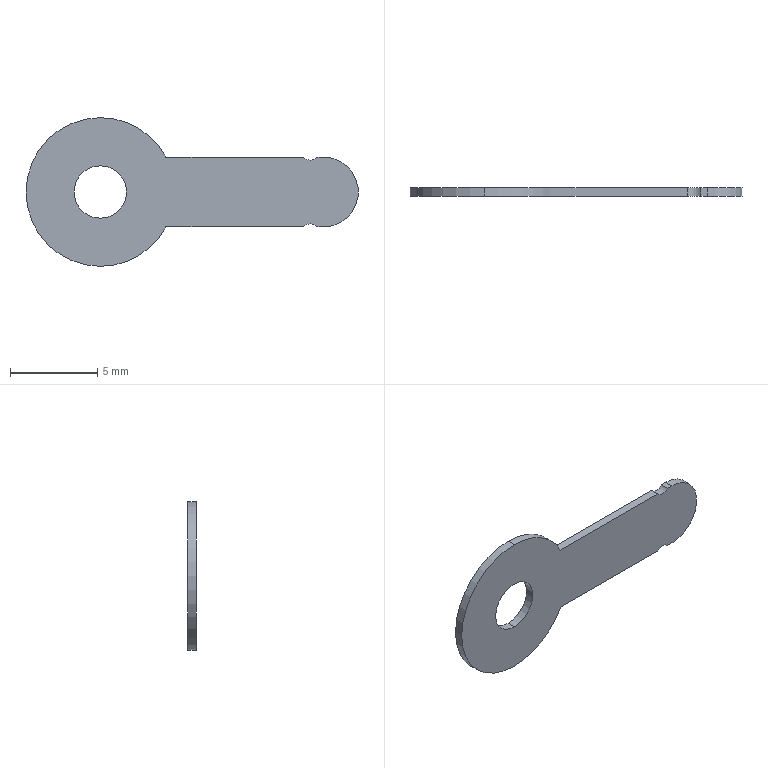Part | SolidWorks | features Extrusion 1, ICE 1 | 1 solid | 15 faces | box 19 x 0.5 x 8.5 mm | volume 45.209 mm3 | cylinder 9 | plane 6 | commonest cylinder face diameters 1 x3 8.5 x3 3 x2 4 x1
STEP:
#1=CARTESIAN_POINT('',(12.,0.,-1.82));
#2=VERTEX_POINT('',#1);
#3=CARTESIAN_POINT('',(12.384,0.,-2.));
#4=VERTEX_POINT('',#3);
#5=CARTESIAN_POINT('',(12.,0.,-2.32));
#6=DIRECTION('',(0.,1.,0.));
#7=DIRECTION('',(0.,0.,1.));
#8=AXIS2_PLACEMENT_3D('',#5,#6,#7);
#9=CIRCLE('',#8,0.5);
#10=EDGE_CURVE('',#2,#4,#9,.T.);
#11=ORIENTED_EDGE('',*,*,#10,.F.);
#12=CARTESIAN_POINT('',(12.,0.5,-1.82));
#13=VERTEX_POINT('',#12);
#14=CARTESIAN_POINT('',(12.,0.,-1.82));
#15=DIRECTION('',(0.,1.,0.));
#16=VECTOR('',#15,1000.);
#17=LINE('',#14,#16);
#18=EDGE_CURVE('',#2,#13,#17,.T.);
#19=ORIENTED_EDGE('',*,*,#18,.T.);
#20=CARTESIAN_POINT('',(12.384,0.5,-2.));
#21=VERTEX_POINT('',#20);
#22=CARTESIAN_POINT('',(12.,0.5,-2.32));
#23=DIRECTION('',(0.,1.,0.));
#24=DIRECTION('',(0.,0.,1.));
#25=AXIS2_PLACEMENT_3D('',#22,#23,#24);
#26=CIRCLE('',#25,0.5);
#27=EDGE_CURVE('',#13,#21,#26,.T.);
#28=ORIENTED_EDGE('',*,*,#27,.T.);
#29=CARTESIAN_POINT('',(12.384,0.,-2.));
#30=DIRECTION('',(0.,1.,0.));
#31=VECTOR('',#30,1000.);
#32=LINE('',#29,#31);
#33=EDGE_CURVE('',#4,#21,#32,.T.);
#34=ORIENTED_EDGE('',*,*,#33,.F.);
#35=EDGE_LOOP('',(#11,#19,#28,#34));
#36=FACE_OUTER_BOUND('',#35,.T.);
#37=CARTESIAN_POINT('',(12.,0.,-2.32));
#38=DIRECTION('',(0.,1.,0.));
#39=DIRECTION('',(0.,0.,1.));
#40=AXIS2_PLACEMENT_3D('',#37,#38,#39);
#41=CYLINDRICAL_SURFACE('',#40,0.5);
#42=ADVANCED_FACE('',(#36),#41,.F.);
#43=CARTESIAN_POINT('',(0.,0.5,-1.5));
#44=VERTEX_POINT('',#43);
#45=CARTESIAN_POINT('',(0.,0.5,1.5));
#46=VERTEX_POINT('',#45);
#47=CARTESIAN_POINT('',(0.,0.5,0.));
#48=DIRECTION('',(0.,1.,0.));
#49=DIRECTION('',(0.,0.,1.));
#50=AXIS2_PLACEMENT_3D('',#47,#48,#49);
#51=CIRCLE('',#50,1.5);
#52=EDGE_CURVE('',#44,#46,#51,.T.);
#53=ORIENTED_EDGE('',*,*,#52,.T.);
#54=CARTESIAN_POINT('',(0.,0.,1.5));
#55=VERTEX_POINT('',#54);
#56=CARTESIAN_POINT('',(0.,0.5,1.5));
#57=DIRECTION('',(0.,-1.,0.));
#58=VECTOR('',#57,1000.);
#59=LINE('',#56,#58);
#60=EDGE_CURVE('',#46,#55,#59,.T.);
#61=ORIENTED_EDGE('',*,*,#60,.T.);
#62=CARTESIAN_POINT('',(0.,0.,-1.5));
#63=VERTEX_POINT('',#62);
#64=CARTESIAN_POINT('',(0.,0.,0.));
#65=DIRECTION('',(0.,1.,0.));
#66=DIRECTION('',(0.,0.,1.));
#67=AXIS2_PLACEMENT_3D('',#64,#65,#66);
#68=CIRCLE('',#67,1.5);
#69=EDGE_CURVE('',#63,#55,#68,.T.);
#70=ORIENTED_EDGE('',*,*,#69,.F.);
#71=CARTESIAN_POINT('',(0.,0.5,-1.5));
#72=DIRECTION('',(0.,-1.,0.));
#73=VECTOR('',#72,1000.);
#74=LINE('',#71,#73);
#75=EDGE_CURVE('',#44,#63,#74,.T.);
#76=ORIENTED_EDGE('',*,*,#75,.F.);
#77=EDGE_LOOP('',(#53,#61,#70,#76));
#78=FACE_OUTER_BOUND('',#77,.T.);
#79=CARTESIAN_POINT('',(0.,0.5,0.));
#80=DIRECTION('',(0.,-1.,0.));
#81=DIRECTION('',(0.,0.,-1.));
#82=AXIS2_PLACEMENT_3D('',#79,#80,#81);
#83=CYLINDRICAL_SURFACE('',#82,1.5);
#84=ADVANCED_FACE('',(#78),#83,.F.);
#85=CARTESIAN_POINT('',(0.,0.5,4.25));
#86=VERTEX_POINT('',#85);
#87=CARTESIAN_POINT('',(3.75,0.5,2.));
#88=VERTEX_POINT('',#87);
#89=CARTESIAN_POINT('',(0.,0.5,0.));
#90=DIRECTION('',(0.,1.,0.));
#91=DIRECTION('',(0.,0.,1.));
#92=AXIS2_PLACEMENT_3D('',#89,#90,#91);
#93=CIRCLE('',#92,4.25);
#94=EDGE_CURVE('',#86,#88,#93,.T.);
#95=ORIENTED_EDGE('',*,*,#94,.F.);
#96=CARTESIAN_POINT('',(0.,0.,4.25));
#97=VERTEX_POINT('',#96);
#98=CARTESIAN_POINT('',(0.,0.5,4.25));
#99=DIRECTION('',(0.,-1.,0.));
#100=VECTOR('',#99,1000.);
#101=LINE('',#98,#100);
#102=EDGE_CURVE('',#86,#97,#101,.T.);
#103=ORIENTED_EDGE('',*,*,#102,.T.);
#104=CARTESIAN_POINT('',(3.75,0.,2.));
#105=VERTEX_POINT('',#104);
#106=CARTESIAN_POINT('',(0.,0.,0.));
#107=DIRECTION('',(0.,1.,0.));
#108=DIRECTION('',(0.,0.,1.));
#109=AXIS2_PLACEMENT_3D('',#106,#107,#108);
#110=CIRCLE('',#109,4.25);
#111=EDGE_CURVE('',#97,#105,#110,.T.);
#112=ORIENTED_EDGE('',*,*,#111,.T.);
#113=CARTESIAN_POINT('',(3.75,0.5,2.));
#114=DIRECTION('',(0.,-1.,0.));
#115=VECTOR('',#114,1000.);
#116=LINE('',#113,#115);
#117=EDGE_CURVE('',#88,#105,#116,.T.);
#118=ORIENTED_EDGE('',*,*,#117,.F.);
#119=EDGE_LOOP('',(#95,#103,#112,#118));
#120=FACE_OUTER_BOUND('',#119,.T.);
#121=CARTESIAN_POINT('',(0.,0.5,0.));
#122=DIRECTION('',(0.,-1.,0.));
#123=DIRECTION('',(0.,0.,-1.));
#124=AXIS2_PLACEMENT_3D('',#121,#122,#123);
#125=CYLINDRICAL_SURFACE('',#124,4.25);
#126=ADVANCED_FACE('',(#120),#125,.T.);
#127=ORIENTED_EDGE('',*,*,#102,.F.);
#128=CARTESIAN_POINT('',(0.,0.5,-4.25));
#129=VERTEX_POINT('',#128);
#130=CARTESIAN_POINT('',(0.,0.5,0.));
#131=DIRECTION('',(0.,1.,0.));
#132=DIRECTION('',(0.,0.,1.));
#133=AXIS2_PLACEMENT_3D('',#130,#131,#132);
#134=CIRCLE('',#133,4.25);
#135=EDGE_CURVE('',#129,#86,#134,.T.);
#136=ORIENTED_EDGE('',*,*,#135,.F.);
#137=CARTESIAN_POINT('',(0.,0.,-4.25));
#138=VERTEX_POINT('',#137);
#139=CARTESIAN_POINT('',(0.,0.5,-4.25));
#140=DIRECTION('',(0.,-1.,0.));
#141=VECTOR('',#140,1000.);
#142=LINE('',#139,#141);
#143=EDGE_CURVE('',#129,#138,#142,.T.);
#144=ORIENTED_EDGE('',*,*,#143,.T.);
#145=CARTESIAN_POINT('',(0.,0.,0.));
#146=DIRECTION('',(0.,1.,0.));
#147=DIRECTION('',(0.,0.,1.));
#148=AXIS2_PLACEMENT_3D('',#145,#146,#147);
#149=CIRCLE('',#148,4.25);
#150=EDGE_CURVE('',#138,#97,#149,.T.);
#151=ORIENTED_EDGE('',*,*,#150,.T.);
#152=EDGE_LOOP('',(#127,#136,#144,#151));
#153=FACE_OUTER_BOUND('',#152,.T.);
#154=CARTESIAN_POINT('',(0.,0.5,0.));
#155=DIRECTION('',(0.,-1.,0.));
#156=DIRECTION('',(0.,0.,-1.));
#157=AXIS2_PLACEMENT_3D('',#154,#155,#156);
#158=CYLINDRICAL_SURFACE('',#157,4.25);
#159=ADVANCED_FACE('',(#153),#158,.T.);
#160=CARTESIAN_POINT('',(11.616,0.,2.));
#161=VERTEX_POINT('',#160);
#162=CARTESIAN_POINT('',(12.75,0.,2.));
#163=DIRECTION('',(1.,0.,0.));
#164=VECTOR('',#163,1000.);
#165=LINE('',#162,#164);
#166=EDGE_CURVE('',#105,#161,#165,.T.);
#167=ORIENTED_EDGE('',*,*,#166,.T.);
#168=CARTESIAN_POINT('',(11.616,0.5,2.));
#169=VERTEX_POINT('',#168);
#170=CARTESIAN_POINT('',(11.616,0.,2.));
#171=DIRECTION('',(0.,1.,0.));
#172=VECTOR('',#171,1000.);
#173=LINE('',#170,#172);
#174=EDGE_CURVE('',#161,#169,#173,.T.);
#175=ORIENTED_EDGE('',*,*,#174,.T.);
#176=CARTESIAN_POINT('',(12.75,0.5,2.));
#177=DIRECTION('',(1.,0.,0.));
#178=VECTOR('',#177,1000.);
#179=LINE('',#176,#178);
#180=EDGE_CURVE('',#88,#169,#179,.T.);
#181=ORIENTED_EDGE('',*,*,#180,.F.);
#182=ORIENTED_EDGE('',*,*,#117,.T.);
#183=EDGE_LOOP('',(#167,#175,#181,#182));
#184=FACE_OUTER_BOUND('',#183,.T.);
#185=CARTESIAN_POINT('',(12.75,0.5,2.));
#186=DIRECTION('',(0.,0.,-1.));
#187=DIRECTION('',(-1.,0.,0.));
#188=AXIS2_PLACEMENT_3D('',#185,#186,#187);
#189=PLANE('',#188);
#190=ADVANCED_FACE('',(#184),#189,.F.);
#191=CARTESIAN_POINT('',(12.75,0.,-2.));
#192=VERTEX_POINT('',#191);
#193=CARTESIAN_POINT('',(12.75,0.,-2.));
#194=DIRECTION('',(-1.,0.,0.));
#195=VECTOR('',#194,1000.);
#196=LINE('',#193,#195);
#197=EDGE_CURVE('',#192,#4,#196,.T.);
#198=ORIENTED_EDGE('',*,*,#197,.T.);
#199=ORIENTED_EDGE('',*,*,#33,.T.);
#200=CARTESIAN_POINT('',(12.75,0.5,-2.));
#201=VERTEX_POINT('',#200);
#202=CARTESIAN_POINT('',(12.75,0.5,-2.));
#203=DIRECTION('',(-1.,0.,0.));
#204=VECTOR('',#203,1000.);
#205=LINE('',#202,#204);
#206=EDGE_CURVE('',#201,#21,#205,.T.);
#207=ORIENTED_EDGE('',*,*,#206,.F.);
#208=CARTESIAN_POINT('',(12.75,0.5,-2.));
#209=DIRECTION('',(0.,-1.,0.));
#210=VECTOR('',#209,1000.);
#211=LINE('',#208,#210);
#212=EDGE_CURVE('',#201,#192,#211,.T.);
#213=ORIENTED_EDGE('',*,*,#212,.T.);
#214=EDGE_LOOP('',(#198,#199,#207,#213));
#215=FACE_OUTER_BOUND('',#214,.T.);
#216=CARTESIAN_POINT('',(12.75,0.5,-2.));
#217=DIRECTION('',(0.,0.,1.));
#218=DIRECTION('',(1.,0.,0.));
#219=AXIS2_PLACEMENT_3D('',#216,#217,#218);
#220=PLANE('',#219);
#221=ADVANCED_FACE('',(#215),#220,.F.);
#222=CARTESIAN_POINT('',(12.384,0.5,2.));
#223=VERTEX_POINT('',#222);
#224=CARTESIAN_POINT('',(12.,0.5,2.32));
#225=DIRECTION('',(0.,1.,0.));
#226=DIRECTION('',(0.,0.,1.));
#227=AXIS2_PLACEMENT_3D('',#224,#225,#226);
#228=CIRCLE('',#227,0.5);
#229=EDGE_CURVE('',#223,#169,#228,.T.);
#230=ORIENTED_EDGE('',*,*,#229,.F.);
#231=CARTESIAN_POINT('',(12.75,0.5,2.));
#232=VERTEX_POINT('',#231);
#233=CARTESIAN_POINT('',(12.75,0.5,2.));
#234=DIRECTION('',(1.,0.,0.));
#235=VECTOR('',#234,1000.);
#236=LINE('',#233,#235);
#237=EDGE_CURVE('',#223,#232,#236,.T.);
#238=ORIENTED_EDGE('',*,*,#237,.T.);
#239=CARTESIAN_POINT('',(12.75,0.5,0.));
#240=DIRECTION('',(0.,1.,0.));
#241=DIRECTION('',(0.,0.,1.));
#242=AXIS2_PLACEMENT_3D('',#239,#240,#241);
#243=CIRCLE('',#242,2.);
#244=EDGE_CURVE('',#232,#201,#243,.T.);
#245=ORIENTED_EDGE('',*,*,#244,.T.);
#246=ORIENTED_EDGE('',*,*,#206,.T.);
#247=ORIENTED_EDGE('',*,*,#27,.F.);
#248=CARTESIAN_POINT('',(11.616,0.5,-2.));
#249=VERTEX_POINT('',#248);
#250=CARTESIAN_POINT('',(12.,0.5,-2.32));
#251=DIRECTION('',(0.,1.,0.));
#252=DIRECTION('',(0.,0.,1.));
#253=AXIS2_PLACEMENT_3D('',#250,#251,#252);
#254=CIRCLE('',#253,0.5);
#255=EDGE_CURVE('',#249,#13,#254,.T.);
#256=ORIENTED_EDGE('',*,*,#255,.F.);
#257=CARTESIAN_POINT('',(3.75,0.5,-2.));
#258=VERTEX_POINT('',#257);
#259=CARTESIAN_POINT('',(12.75,0.5,-2.));
#260=DIRECTION('',(-1.,0.,0.));
#261=VECTOR('',#260,1000.);
#262=LINE('',#259,#261);
#263=EDGE_CURVE('',#249,#258,#262,.T.);
#264=ORIENTED_EDGE('',*,*,#263,.T.);
#265=CARTESIAN_POINT('',(0.,0.5,0.));
#266=DIRECTION('',(0.,1.,0.));
#267=DIRECTION('',(0.,0.,1.));
#268=AXIS2_PLACEMENT_3D('',#265,#266,#267);
#269=CIRCLE('',#268,4.25);
#270=EDGE_CURVE('',#258,#129,#269,.T.);
#271=ORIENTED_EDGE('',*,*,#270,.T.);
#272=ORIENTED_EDGE('',*,*,#135,.T.);
#273=ORIENTED_EDGE('',*,*,#94,.T.);
#274=ORIENTED_EDGE('',*,*,#180,.T.);
#275=EDGE_LOOP('',(#230,#238,#245,#246,#247,#256,#264,#271,#272,#273,#274));
#276=FACE_OUTER_BOUND('',#275,.T.);
#277=ORIENTED_EDGE('',*,*,#52,.F.);
#278=CARTESIAN_POINT('',(0.,0.5,0.));
#279=DIRECTION('',(0.,1.,0.));
#280=DIRECTION('',(0.,0.,1.));
#281=AXIS2_PLACEMENT_3D('',#278,#279,#280);
#282=CIRCLE('',#281,1.5);
#283=EDGE_CURVE('',#46,#44,#282,.T.);
#284=ORIENTED_EDGE('',*,*,#283,.F.);
#285=EDGE_LOOP('',(#277,#284));
#286=FACE_BOUND('',#285,.T.);
#287=CARTESIAN_POINT('',(12.75,0.5,0.));
#288=DIRECTION('',(0.,1.,0.));
#289=DIRECTION('',(0.,0.,1.));
#290=AXIS2_PLACEMENT_3D('',#287,#288,#289);
#291=PLANE('',#290);
#292=ADVANCED_FACE('',(#276,#286),#291,.T.);
#293=CARTESIAN_POINT('',(12.384,0.,2.));
#294=VERTEX_POINT('',#293);
#295=CARTESIAN_POINT('',(12.75,0.,2.));
#296=VERTEX_POINT('',#295);
#297=CARTESIAN_POINT('',(12.75,0.,2.));
#298=DIRECTION('',(1.,0.,0.));
#299=VECTOR('',#298,1000.);
#300=LINE('',#297,#299);
#301=EDGE_CURVE('',#294,#296,#300,.T.);
#302=ORIENTED_EDGE('',*,*,#301,.F.);
#303=CARTESIAN_POINT('',(12.,0.,2.32));
#304=DIRECTION('',(0.,1.,0.));
#305=DIRECTION('',(0.,0.,1.));
#306=AXIS2_PLACEMENT_3D('',#303,#304,#305);
#307=CIRCLE('',#306,0.5);
#308=EDGE_CURVE('',#294,#161,#307,.T.);
#309=ORIENTED_EDGE('',*,*,#308,.T.);
#310=ORIENTED_EDGE('',*,*,#166,.F.);
#311=ORIENTED_EDGE('',*,*,#111,.F.);
#312=ORIENTED_EDGE('',*,*,#150,.F.);
#313=CARTESIAN_POINT('',(3.75,0.,-2.));
#314=VERTEX_POINT('',#313);
#315=CARTESIAN_POINT('',(0.,0.,0.));
#316=DIRECTION('',(0.,1.,0.));
#317=DIRECTION('',(0.,0.,1.));
#318=AXIS2_PLACEMENT_3D('',#315,#316,#317);
#319=CIRCLE('',#318,4.25);
#320=EDGE_CURVE('',#314,#138,#319,.T.);
#321=ORIENTED_EDGE('',*,*,#320,.F.);
#322=CARTESIAN_POINT('',(11.616,0.,-2.));
#323=VERTEX_POINT('',#322);
#324=CARTESIAN_POINT('',(12.75,0.,-2.));
#325=DIRECTION('',(-1.,0.,0.));
#326=VECTOR('',#325,1000.);
#327=LINE('',#324,#326);
#328=EDGE_CURVE('',#323,#314,#327,.T.);
#329=ORIENTED_EDGE('',*,*,#328,.F.);
#330=CARTESIAN_POINT('',(12.,0.,-2.32));
#331=DIRECTION('',(0.,1.,0.));
#332=DIRECTION('',(0.,0.,1.));
#333=AXIS2_PLACEMENT_3D('',#330,#331,#332);
#334=CIRCLE('',#333,0.5);
#335=EDGE_CURVE('',#323,#2,#334,.T.);
#336=ORIENTED_EDGE('',*,*,#335,.T.);
#337=ORIENTED_EDGE('',*,*,#10,.T.);
#338=ORIENTED_EDGE('',*,*,#197,.F.);
#339=CARTESIAN_POINT('',(12.75,0.,0.));
#340=DIRECTION('',(0.,1.,0.));
#341=DIRECTION('',(0.,0.,1.));
#342=AXIS2_PLACEMENT_3D('',#339,#340,#341);
#343=CIRCLE('',#342,2.);
#344=EDGE_CURVE('',#296,#192,#343,.T.);
#345=ORIENTED_EDGE('',*,*,#344,.F.);
#346=EDGE_LOOP('',(#302,#309,#310,#311,#312,#321,#329,#336,#337,#338,#345));
#347=FACE_OUTER_BOUND('',#346,.T.);
#348=ORIENTED_EDGE('',*,*,#69,.T.);
#349=CARTESIAN_POINT('',(0.,0.,0.));
#350=DIRECTION('',(0.,1.,0.));
#351=DIRECTION('',(0.,0.,1.));
#352=AXIS2_PLACEMENT_3D('',#349,#350,#351);
#353=CIRCLE('',#352,1.5);
#354=EDGE_CURVE('',#55,#63,#353,.T.);
#355=ORIENTED_EDGE('',*,*,#354,.T.);
#356=EDGE_LOOP('',(#348,#355));
#357=FACE_BOUND('',#356,.T.);
#358=CARTESIAN_POINT('',(12.75,0.,0.));
#359=DIRECTION('',(0.,1.,0.));
#360=DIRECTION('',(0.,0.,1.));
#361=AXIS2_PLACEMENT_3D('',#358,#359,#360);
#362=PLANE('',#361);
#363=ADVANCED_FACE('',(#347,#357),#362,.F.);
#364=ORIENTED_EDGE('',*,*,#344,.T.);
#365=ORIENTED_EDGE('',*,*,#212,.F.);
#366=ORIENTED_EDGE('',*,*,#244,.F.);
#367=CARTESIAN_POINT('',(12.75,0.5,2.));
#368=DIRECTION('',(0.,-1.,0.));
#369=VECTOR('',#368,1000.);
#370=LINE('',#367,#369);
#371=EDGE_CURVE('',#232,#296,#370,.T.);
#372=ORIENTED_EDGE('',*,*,#371,.T.);
#373=EDGE_LOOP('',(#364,#365,#366,#372));
#374=FACE_OUTER_BOUND('',#373,.T.);
#375=CARTESIAN_POINT('',(12.75,0.5,0.));
#376=DIRECTION('',(0.,-1.,0.));
#377=DIRECTION('',(0.,0.,-1.));
#378=AXIS2_PLACEMENT_3D('',#375,#376,#377);
#379=CYLINDRICAL_SURFACE('',#378,2.);
#380=ADVANCED_FACE('',(#374),#379,.T.);
#381=ORIENTED_EDGE('',*,*,#263,.F.);
#382=CARTESIAN_POINT('',(11.616,0.,-2.));
#383=DIRECTION('',(0.,-1.,0.));
#384=VECTOR('',#383,1000.);
#385=LINE('',#382,#384);
#386=EDGE_CURVE('',#249,#323,#385,.T.);
#387=ORIENTED_EDGE('',*,*,#386,.T.);
#388=ORIENTED_EDGE('',*,*,#328,.T.);
#389=CARTESIAN_POINT('',(3.75,0.5,-2.));
#390=DIRECTION('',(0.,-1.,0.));
#391=VECTOR('',#390,1000.);
#392=LINE('',#389,#391);
#393=EDGE_CURVE('',#258,#314,#392,.T.);
#394=ORIENTED_EDGE('',*,*,#393,.F.);
#395=EDGE_LOOP('',(#381,#387,#388,#394));
#396=FACE_OUTER_BOUND('',#395,.T.);
#397=CARTESIAN_POINT('',(12.75,0.5,-2.));
#398=DIRECTION('',(0.,0.,1.));
#399=DIRECTION('',(1.,0.,0.));
#400=AXIS2_PLACEMENT_3D('',#397,#398,#399);
#401=PLANE('',#400);
#402=ADVANCED_FACE('',(#396),#401,.F.);
#403=ORIENTED_EDGE('',*,*,#143,.F.);
#404=ORIENTED_EDGE('',*,*,#270,.F.);
#405=ORIENTED_EDGE('',*,*,#393,.T.);
#406=ORIENTED_EDGE('',*,*,#320,.T.);
#407=EDGE_LOOP('',(#403,#404,#405,#406));
#408=FACE_OUTER_BOUND('',#407,.T.);
#409=CARTESIAN_POINT('',(0.,0.5,0.));
#410=DIRECTION('',(0.,-1.,0.));
#411=DIRECTION('',(0.,0.,-1.));
#412=AXIS2_PLACEMENT_3D('',#409,#410,#411);
#413=CYLINDRICAL_SURFACE('',#412,4.25);
#414=ADVANCED_FACE('',(#408),#413,.T.);
#415=ORIENTED_EDGE('',*,*,#237,.F.);
#416=CARTESIAN_POINT('',(12.384,0.,2.));
#417=DIRECTION('',(0.,-1.,0.));
#418=VECTOR('',#417,1000.);
#419=LINE('',#416,#418);
#420=EDGE_CURVE('',#223,#294,#419,.T.);
#421=ORIENTED_EDGE('',*,*,#420,.T.);
#422=ORIENTED_EDGE('',*,*,#301,.T.);
#423=ORIENTED_EDGE('',*,*,#371,.F.);
#424=EDGE_LOOP('',(#415,#421,#422,#423));
#425=FACE_OUTER_BOUND('',#424,.T.);
#426=CARTESIAN_POINT('',(12.75,0.5,2.));
#427=DIRECTION('',(0.,0.,-1.));
#428=DIRECTION('',(-1.,0.,0.));
#429=AXIS2_PLACEMENT_3D('',#426,#427,#428);
#430=PLANE('',#429);
#431=ADVANCED_FACE('',(#425),#430,.F.);
#432=ORIENTED_EDGE('',*,*,#60,.F.);
#433=ORIENTED_EDGE('',*,*,#283,.T.);
#434=ORIENTED_EDGE('',*,*,#75,.T.);
#435=ORIENTED_EDGE('',*,*,#354,.F.);
#436=EDGE_LOOP('',(#432,#433,#434,#435));
#437=FACE_OUTER_BOUND('',#436,.T.);
#438=CARTESIAN_POINT('',(0.,0.5,0.));
#439=DIRECTION('',(0.,-1.,0.));
#440=DIRECTION('',(0.,0.,-1.));
#441=AXIS2_PLACEMENT_3D('',#438,#439,#440);
#442=CYLINDRICAL_SURFACE('',#441,1.5);
#443=ADVANCED_FACE('',(#437),#442,.F.);
#444=ORIENTED_EDGE('',*,*,#18,.F.);
#445=ORIENTED_EDGE('',*,*,#335,.F.);
#446=ORIENTED_EDGE('',*,*,#386,.F.);
#447=ORIENTED_EDGE('',*,*,#255,.T.);
#448=EDGE_LOOP('',(#444,#445,#446,#447));
#449=FACE_OUTER_BOUND('',#448,.T.);
#450=CARTESIAN_POINT('',(12.,0.,-2.32));
#451=DIRECTION('',(0.,1.,0.));
#452=DIRECTION('',(0.,0.,1.));
#453=AXIS2_PLACEMENT_3D('',#450,#451,#452);
#454=CYLINDRICAL_SURFACE('',#453,0.5);
#455=ADVANCED_FACE('',(#449),#454,.F.);
#456=ORIENTED_EDGE('',*,*,#308,.F.);
#457=ORIENTED_EDGE('',*,*,#420,.F.);
#458=ORIENTED_EDGE('',*,*,#229,.T.);
#459=ORIENTED_EDGE('',*,*,#174,.F.);
#460=EDGE_LOOP('',(#456,#457,#458,#459));
#461=FACE_OUTER_BOUND('',#460,.T.);
#462=CARTESIAN_POINT('',(12.,0.,2.32));
#463=DIRECTION('',(0.,1.,0.));
#464=DIRECTION('',(0.,0.,1.));
#465=AXIS2_PLACEMENT_3D('',#462,#463,#464);
#466=CYLINDRICAL_SURFACE('',#465,0.5);
#467=ADVANCED_FACE('',(#461),#466,.F.);
#468=CLOSED_SHELL('',(#42,#84,#126,#159,#190,#221,#292,#363,#380,#402,#414,#431,#443,#455,#467));
#469=MANIFOLD_SOLID_BREP('',#468);
#470=CARTESIAN_POINT('',(0.,0.,0.));
#471=DIRECTION('',(0.,0.,1.));
#472=DIRECTION('',(1.,0.,0.));
#473=AXIS2_PLACEMENT_3D('',#470,#471,#472);
#474=(LENGTH_UNIT()NAMED_UNIT(*)SI_UNIT(.MILLI.,.METRE.));
#475=UNCERTAINTY_MEASURE_WITH_UNIT(LENGTH_MEASURE(0.00001),#474,'','');
#476=(NAMED_UNIT(*)PLANE_ANGLE_UNIT()SI_UNIT($,.RADIAN.));
#477=(NAMED_UNIT(*)SI_UNIT($,.STERADIAN.)SOLID_ANGLE_UNIT());
#478=(GEOMETRIC_REPRESENTATION_CONTEXT(3)GLOBAL_UNCERTAINTY_ASSIGNED_CONTEXT((#475))GLOBAL_UNIT_ASSIGNED_CONTEXT((#474,#476,#477))REPRESENTATION_CONTEXT('',''));
#479=ADVANCED_BREP_SHAPE_REPRESENTATION('',(#469,#473),#478);